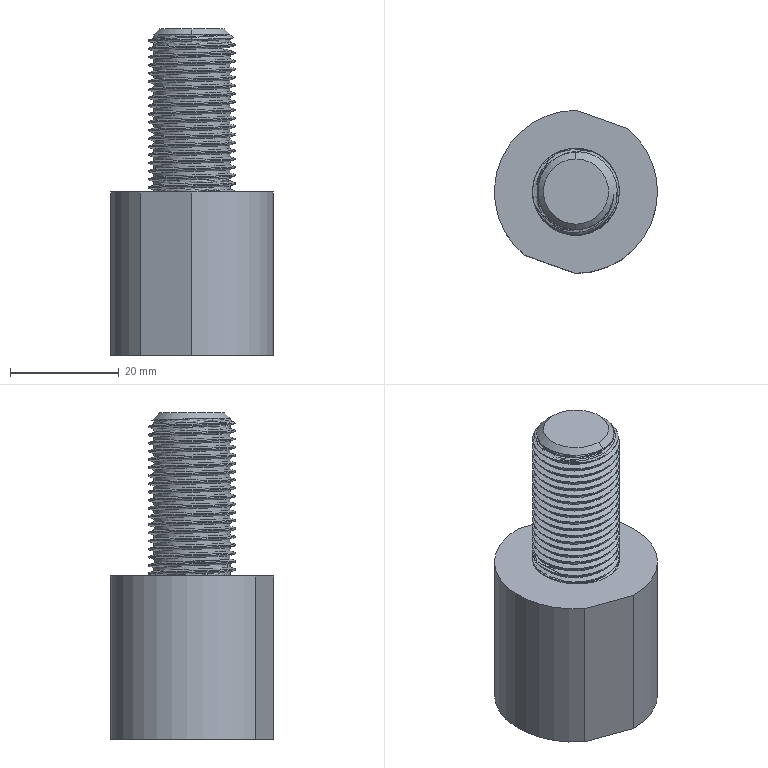Part | SolidWorks | features BaseBody 1 | 1 solid | 57 faces | box 30 x 30 x 60 mm | volume 22398 mm3 | cylinder 44 | cone 5 | plane 5 | spline 3 | commonest cylinder face diameters 16 x39 30 x3 14.5 x2